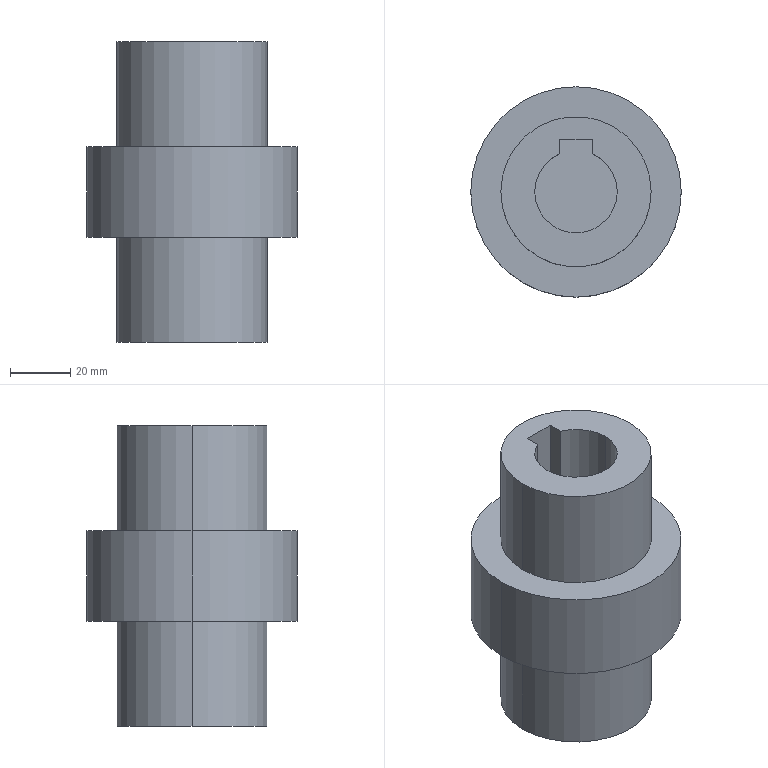Part | SolidWorks | features ICE 5, Extrusion 1 | 1 solid | 24 faces | box 70 x 70 x 100 mm | volume 224245 mm3 | plane 13 | cylinder 11 | commonest cylinder face diameters 50 x4 27.5 x3 25 x2 70 x2
STEP:
#1=CARTESIAN_POINT('',(-13.75,0.,25.));
#2=VERTEX_POINT('',#1);
#3=CARTESIAN_POINT('',(13.75,0.,25.));
#4=VERTEX_POINT('',#3);
#5=CARTESIAN_POINT('',(0.,0.,25.));
#6=DIRECTION('',(0.,0.,1.));
#7=DIRECTION('',(1.,0.,0.));
#8=AXIS2_PLACEMENT_3D('',#5,#6,#7);
#9=CIRCLE('',#8,13.75);
#10=EDGE_CURVE('',#2,#4,#9,.T.);
#11=ORIENTED_EDGE('',*,*,#10,.F.);
#12=CARTESIAN_POINT('',(-13.75,0.,50.));
#13=VERTEX_POINT('',#12);
#14=CARTESIAN_POINT('',(-13.75,0.,25.));
#15=DIRECTION('',(0.,0.,1.));
#16=VECTOR('',#15,1000.);
#17=LINE('',#14,#16);
#18=EDGE_CURVE('',#2,#13,#17,.T.);
#19=ORIENTED_EDGE('',*,*,#18,.T.);
#20=CARTESIAN_POINT('',(13.75,0.,50.));
#21=VERTEX_POINT('',#20);
#22=CARTESIAN_POINT('',(0.,0.,50.));
#23=DIRECTION('',(0.,0.,1.));
#24=DIRECTION('',(1.,0.,0.));
#25=AXIS2_PLACEMENT_3D('',#22,#23,#24);
#26=CIRCLE('',#25,13.75);
#27=EDGE_CURVE('',#13,#21,#26,.T.);
#28=ORIENTED_EDGE('',*,*,#27,.T.);
#29=CARTESIAN_POINT('',(13.75,0.,25.));
#30=DIRECTION('',(0.,0.,1.));
#31=VECTOR('',#30,1000.);
#32=LINE('',#29,#31);
#33=EDGE_CURVE('',#4,#21,#32,.T.);
#34=ORIENTED_EDGE('',*,*,#33,.F.);
#35=EDGE_LOOP('',(#11,#19,#28,#34));
#36=FACE_OUTER_BOUND('',#35,.T.);
#37=CARTESIAN_POINT('',(0.,0.,25.));
#38=DIRECTION('',(0.,0.,1.));
#39=DIRECTION('',(1.,0.,0.));
#40=AXIS2_PLACEMENT_3D('',#37,#38,#39);
#41=CYLINDRICAL_SURFACE('',#40,13.75);
#42=ADVANCED_FACE('',(#36),#41,.F.);
#43=CARTESIAN_POINT('',(5.385,12.652,25.));
#44=VERTEX_POINT('',#43);
#45=CARTESIAN_POINT('',(0.,0.,25.));
#46=DIRECTION('',(0.,0.,1.));
#47=DIRECTION('',(1.,0.,0.));
#48=AXIS2_PLACEMENT_3D('',#45,#46,#47);
#49=CIRCLE('',#48,13.75);
#50=EDGE_CURVE('',#4,#44,#49,.T.);
#51=ORIENTED_EDGE('',*,*,#50,.F.);
#52=ORIENTED_EDGE('',*,*,#33,.T.);
#53=CARTESIAN_POINT('',(5.385,12.652,50.));
#54=VERTEX_POINT('',#53);
#55=CARTESIAN_POINT('',(0.,0.,50.));
#56=DIRECTION('',(0.,0.,1.));
#57=DIRECTION('',(1.,0.,0.));
#58=AXIS2_PLACEMENT_3D('',#55,#56,#57);
#59=CIRCLE('',#58,13.75);
#60=EDGE_CURVE('',#21,#54,#59,.T.);
#61=ORIENTED_EDGE('',*,*,#60,.T.);
#62=CARTESIAN_POINT('',(5.385,12.652,25.));
#63=DIRECTION('',(0.,0.,1.));
#64=VECTOR('',#63,1000.);
#65=LINE('',#62,#64);
#66=EDGE_CURVE('',#44,#54,#65,.T.);
#67=ORIENTED_EDGE('',*,*,#66,.F.);
#68=EDGE_LOOP('',(#51,#52,#61,#67));
#69=FACE_OUTER_BOUND('',#68,.T.);
#70=CARTESIAN_POINT('',(0.,0.,25.));
#71=DIRECTION('',(0.,0.,1.));
#72=DIRECTION('',(1.,0.,0.));
#73=AXIS2_PLACEMENT_3D('',#70,#71,#72);
#74=CYLINDRICAL_SURFACE('',#73,13.75);
#75=ADVANCED_FACE('',(#69),#74,.F.);
#76=CARTESIAN_POINT('',(-25.,0.,-50.));
#77=VERTEX_POINT('',#76);
#78=CARTESIAN_POINT('',(25.,0.,-50.));
#79=VERTEX_POINT('',#78);
#80=CARTESIAN_POINT('',(0.,0.,-50.));
#81=DIRECTION('',(0.,0.,-1.));
#82=DIRECTION('',(-1.,0.,0.));
#83=AXIS2_PLACEMENT_3D('',#80,#81,#82);
#84=CIRCLE('',#83,25.);
#85=EDGE_CURVE('',#77,#79,#84,.T.);
#86=ORIENTED_EDGE('',*,*,#85,.F.);
#87=CARTESIAN_POINT('',(-25.,0.,-15.));
#88=VERTEX_POINT('',#87);
#89=CARTESIAN_POINT('',(-25.,0.,-50.));
#90=DIRECTION('',(0.,0.,1.));
#91=VECTOR('',#90,1000.);
#92=LINE('',#89,#91);
#93=EDGE_CURVE('',#77,#88,#92,.T.);
#94=ORIENTED_EDGE('',*,*,#93,.T.);
#95=CARTESIAN_POINT('',(25.,0.,-15.));
#96=VERTEX_POINT('',#95);
#97=CARTESIAN_POINT('',(0.,0.,-15.));
#98=DIRECTION('',(0.,0.,-1.));
#99=DIRECTION('',(-1.,0.,0.));
#100=AXIS2_PLACEMENT_3D('',#97,#98,#99);
#101=CIRCLE('',#100,25.);
#102=EDGE_CURVE('',#88,#96,#101,.T.);
#103=ORIENTED_EDGE('',*,*,#102,.T.);
#104=CARTESIAN_POINT('',(25.,0.,-50.));
#105=DIRECTION('',(0.,0.,1.));
#106=VECTOR('',#105,1000.);
#107=LINE('',#104,#106);
#108=EDGE_CURVE('',#79,#96,#107,.T.);
#109=ORIENTED_EDGE('',*,*,#108,.F.);
#110=EDGE_LOOP('',(#86,#94,#103,#109));
#111=FACE_OUTER_BOUND('',#110,.T.);
#112=CARTESIAN_POINT('',(0.,0.,-50.));
#113=DIRECTION('',(0.,0.,1.));
#114=DIRECTION('',(1.,0.,0.));
#115=AXIS2_PLACEMENT_3D('',#112,#113,#114);
#116=CYLINDRICAL_SURFACE('',#115,25.);
#117=ADVANCED_FACE('',(#111),#116,.T.);
#118=CARTESIAN_POINT('',(25.,0.,50.));
#119=VERTEX_POINT('',#118);
#120=CARTESIAN_POINT('',(-25.,0.,50.));
#121=VERTEX_POINT('',#120);
#122=CARTESIAN_POINT('',(0.,0.,50.));
#123=DIRECTION('',(0.,0.,1.));
#124=DIRECTION('',(1.,0.,0.));
#125=AXIS2_PLACEMENT_3D('',#122,#123,#124);
#126=CIRCLE('',#125,25.);
#127=EDGE_CURVE('',#119,#121,#126,.T.);
#128=ORIENTED_EDGE('',*,*,#127,.F.);
#129=CARTESIAN_POINT('',(25.,0.,15.));
#130=VERTEX_POINT('',#129);
#131=CARTESIAN_POINT('',(25.,0.,50.));
#132=DIRECTION('',(0.,0.,-1.));
#133=VECTOR('',#132,1000.);
#134=LINE('',#131,#133);
#135=EDGE_CURVE('',#119,#130,#134,.T.);
#136=ORIENTED_EDGE('',*,*,#135,.T.);
#137=CARTESIAN_POINT('',(-25.,0.,15.));
#138=VERTEX_POINT('',#137);
#139=CARTESIAN_POINT('',(0.,0.,15.));
#140=DIRECTION('',(0.,0.,1.));
#141=DIRECTION('',(1.,0.,0.));
#142=AXIS2_PLACEMENT_3D('',#139,#140,#141);
#143=CIRCLE('',#142,25.);
#144=EDGE_CURVE('',#130,#138,#143,.T.);
#145=ORIENTED_EDGE('',*,*,#144,.T.);
#146=CARTESIAN_POINT('',(-25.,0.,50.));
#147=DIRECTION('',(0.,0.,-1.));
#148=VECTOR('',#147,1000.);
#149=LINE('',#146,#148);
#150=EDGE_CURVE('',#121,#138,#149,.T.);
#151=ORIENTED_EDGE('',*,*,#150,.F.);
#152=EDGE_LOOP('',(#128,#136,#145,#151));
#153=FACE_OUTER_BOUND('',#152,.T.);
#154=CARTESIAN_POINT('',(0.,0.,50.));
#155=DIRECTION('',(0.,0.,-1.));
#156=DIRECTION('',(-1.,0.,0.));
#157=AXIS2_PLACEMENT_3D('',#154,#155,#156);
#158=CYLINDRICAL_SURFACE('',#157,25.);
#159=ADVANCED_FACE('',(#153),#158,.T.);
#160=CARTESIAN_POINT('',(35.,0.,15.));
#161=VERTEX_POINT('',#160);
#162=CARTESIAN_POINT('',(-35.,0.,15.));
#163=VERTEX_POINT('',#162);
#164=CARTESIAN_POINT('',(0.,0.,15.));
#165=DIRECTION('',(0.,0.,1.));
#166=DIRECTION('',(1.,0.,0.));
#167=AXIS2_PLACEMENT_3D('',#164,#165,#166);
#168=CIRCLE('',#167,35.);
#169=EDGE_CURVE('',#161,#163,#168,.T.);
#170=ORIENTED_EDGE('',*,*,#169,.F.);
#171=CARTESIAN_POINT('',(35.,0.,-15.));
#172=VERTEX_POINT('',#171);
#173=CARTESIAN_POINT('',(35.,0.,15.));
#174=DIRECTION('',(0.,0.,-1.));
#175=VECTOR('',#174,1000.);
#176=LINE('',#173,#175);
#177=EDGE_CURVE('',#161,#172,#176,.T.);
#178=ORIENTED_EDGE('',*,*,#177,.T.);
#179=CARTESIAN_POINT('',(-35.,0.,-15.));
#180=VERTEX_POINT('',#179);
#181=CARTESIAN_POINT('',(0.,0.,-15.));
#182=DIRECTION('',(0.,0.,1.));
#183=DIRECTION('',(1.,0.,0.));
#184=AXIS2_PLACEMENT_3D('',#181,#182,#183);
#185=CIRCLE('',#184,35.);
#186=EDGE_CURVE('',#172,#180,#185,.T.);
#187=ORIENTED_EDGE('',*,*,#186,.T.);
#188=CARTESIAN_POINT('',(-35.,0.,15.));
#189=DIRECTION('',(0.,0.,-1.));
#190=VECTOR('',#189,1000.);
#191=LINE('',#188,#190);
#192=EDGE_CURVE('',#163,#180,#191,.T.);
#193=ORIENTED_EDGE('',*,*,#192,.F.);
#194=EDGE_LOOP('',(#170,#178,#187,#193));
#195=FACE_OUTER_BOUND('',#194,.T.);
#196=CARTESIAN_POINT('',(0.,0.,15.));
#197=DIRECTION('',(0.,0.,-1.));
#198=DIRECTION('',(-1.,0.,0.));
#199=AXIS2_PLACEMENT_3D('',#196,#197,#198);
#200=CYLINDRICAL_SURFACE('',#199,35.);
#201=ADVANCED_FACE('',(#195),#200,.T.);
#202=CARTESIAN_POINT('',(12.5,0.,-25.));
#203=VERTEX_POINT('',#202);
#204=CARTESIAN_POINT('',(-12.5,0.,-25.));
#205=VERTEX_POINT('',#204);
#206=CARTESIAN_POINT('',(0.,0.,-25.));
#207=DIRECTION('',(0.,0.,-1.));
#208=DIRECTION('',(-1.,0.,0.));
#209=AXIS2_PLACEMENT_3D('',#206,#207,#208);
#210=CIRCLE('',#209,12.5);
#211=EDGE_CURVE('',#203,#205,#210,.T.);
#212=ORIENTED_EDGE('',*,*,#211,.F.);
#213=CARTESIAN_POINT('',(12.5,0.,-50.));
#214=VERTEX_POINT('',#213);
#215=CARTESIAN_POINT('',(12.5,0.,-25.));
#216=DIRECTION('',(0.,0.,-1.));
#217=VECTOR('',#216,1000.);
#218=LINE('',#215,#217);
#219=EDGE_CURVE('',#203,#214,#218,.T.);
#220=ORIENTED_EDGE('',*,*,#219,.T.);
#221=CARTESIAN_POINT('',(-12.5,0.,-50.));
#222=VERTEX_POINT('',#221);
#223=CARTESIAN_POINT('',(0.,0.,-50.));
#224=DIRECTION('',(0.,0.,-1.));
#225=DIRECTION('',(-1.,0.,0.));
#226=AXIS2_PLACEMENT_3D('',#223,#224,#225);
#227=CIRCLE('',#226,12.5);
#228=EDGE_CURVE('',#214,#222,#227,.T.);
#229=ORIENTED_EDGE('',*,*,#228,.T.);
#230=CARTESIAN_POINT('',(-12.5,0.,-25.));
#231=DIRECTION('',(0.,0.,-1.));
#232=VECTOR('',#231,1000.);
#233=LINE('',#230,#232);
#234=EDGE_CURVE('',#205,#222,#233,.T.);
#235=ORIENTED_EDGE('',*,*,#234,.F.);
#236=EDGE_LOOP('',(#212,#220,#229,#235));
#237=FACE_OUTER_BOUND('',#236,.T.);
#238=CARTESIAN_POINT('',(0.,0.,-25.));
#239=DIRECTION('',(0.,0.,-1.));
#240=DIRECTION('',(-1.,0.,0.));
#241=AXIS2_PLACEMENT_3D('',#238,#239,#240);
#242=CYLINDRICAL_SURFACE('',#241,12.5);
#243=ADVANCED_FACE('',(#237),#242,.F.);
#244=CARTESIAN_POINT('',(0.,0.,-50.));
#245=DIRECTION('',(0.,0.,-1.));
#246=DIRECTION('',(-1.,0.,0.));
#247=AXIS2_PLACEMENT_3D('',#244,#245,#246);
#248=CIRCLE('',#247,25.);
#249=EDGE_CURVE('',#79,#77,#248,.T.);
#250=ORIENTED_EDGE('',*,*,#249,.T.);
#251=ORIENTED_EDGE('',*,*,#85,.T.);
#252=EDGE_LOOP('',(#250,#251));
#253=FACE_OUTER_BOUND('',#252,.T.);
#254=CARTESIAN_POINT('',(5.,15.,-50.));
#255=VERTEX_POINT('',#254);
#256=CARTESIAN_POINT('',(-5.,15.,-50.));
#257=VERTEX_POINT('',#256);
#258=CARTESIAN_POINT('',(0.,15.,-50.));
#259=DIRECTION('',(-1.,0.,0.));
#260=VECTOR('',#259,1000.);
#261=LINE('',#258,#260);
#262=EDGE_CURVE('',#255,#257,#261,.T.);
#263=ORIENTED_EDGE('',*,*,#262,.T.);
#264=CARTESIAN_POINT('',(-5.,11.456,-50.));
#265=VERTEX_POINT('',#264);
#266=CARTESIAN_POINT('',(-5.,0.,-50.));
#267=DIRECTION('',(0.,-1.,0.));
#268=VECTOR('',#267,1000.);
#269=LINE('',#266,#268);
#270=EDGE_CURVE('',#257,#265,#269,.T.);
#271=ORIENTED_EDGE('',*,*,#270,.T.);
#272=CARTESIAN_POINT('',(0.,0.,-50.));
#273=DIRECTION('',(0.,0.,-1.));
#274=DIRECTION('',(-1.,0.,0.));
#275=AXIS2_PLACEMENT_3D('',#272,#273,#274);
#276=CIRCLE('',#275,12.5);
#277=EDGE_CURVE('',#222,#265,#276,.T.);
#278=ORIENTED_EDGE('',*,*,#277,.F.);
#279=ORIENTED_EDGE('',*,*,#228,.F.);
#280=CARTESIAN_POINT('',(5.,11.456,-50.));
#281=VERTEX_POINT('',#280);
#282=CARTESIAN_POINT('',(0.,0.,-50.));
#283=DIRECTION('',(0.,0.,-1.));
#284=DIRECTION('',(-1.,0.,0.));
#285=AXIS2_PLACEMENT_3D('',#282,#283,#284);
#286=CIRCLE('',#285,12.5);
#287=EDGE_CURVE('',#281,#214,#286,.T.);
#288=ORIENTED_EDGE('',*,*,#287,.F.);
#289=CARTESIAN_POINT('',(5.,0.,-50.));
#290=DIRECTION('',(0.,-1.,0.));
#291=VECTOR('',#290,1000.);
#292=LINE('',#289,#291);
#293=EDGE_CURVE('',#255,#281,#292,.T.);
#294=ORIENTED_EDGE('',*,*,#293,.F.);
#295=EDGE_LOOP('',(#263,#271,#278,#279,#288,#294));
#296=FACE_BOUND('',#295,.T.);
#297=CARTESIAN_POINT('',(0.,0.,-50.));
#298=DIRECTION('',(0.,0.,-1.));
#299=DIRECTION('',(-1.,0.,0.));
#300=AXIS2_PLACEMENT_3D('',#297,#298,#299);
#301=PLANE('',#300);
#302=ADVANCED_FACE('',(#253,#296),#301,.T.);
#303=ORIENTED_EDGE('',*,*,#219,.F.);
#304=CARTESIAN_POINT('',(0.,0.,-25.));
#305=DIRECTION('',(0.,0.,-1.));
#306=DIRECTION('',(-1.,0.,0.));
#307=AXIS2_PLACEMENT_3D('',#304,#305,#306);
#308=CIRCLE('',#307,12.5);
#309=EDGE_CURVE('',#205,#203,#308,.T.);
#310=ORIENTED_EDGE('',*,*,#309,.F.);
#311=ORIENTED_EDGE('',*,*,#234,.T.);
#312=ORIENTED_EDGE('',*,*,#277,.T.);
#313=CARTESIAN_POINT('',(-5.,11.456,-35.));
#314=VERTEX_POINT('',#313);
#315=CARTESIAN_POINT('',(-5.,11.456,-35.));
#316=DIRECTION('',(0.,0.,-1.));
#317=VECTOR('',#316,1000.);
#318=LINE('',#315,#317);
#319=EDGE_CURVE('',#314,#265,#318,.T.);
#320=ORIENTED_EDGE('',*,*,#319,.F.);
#321=CARTESIAN_POINT('',(5.,11.456,-35.));
#322=VERTEX_POINT('',#321);
#323=CARTESIAN_POINT('',(0.,0.,-35.));
#324=DIRECTION('',(0.,0.,-1.));
#325=DIRECTION('',(-1.,0.,0.));
#326=AXIS2_PLACEMENT_3D('',#323,#324,#325);
#327=CIRCLE('',#326,12.5);
#328=EDGE_CURVE('',#314,#322,#327,.T.);
#329=ORIENTED_EDGE('',*,*,#328,.T.);
#330=CARTESIAN_POINT('',(5.,11.456,-35.));
#331=DIRECTION('',(0.,0.,-1.));
#332=VECTOR('',#331,1000.);
#333=LINE('',#330,#332);
#334=EDGE_CURVE('',#322,#281,#333,.T.);
#335=ORIENTED_EDGE('',*,*,#334,.T.);
#336=ORIENTED_EDGE('',*,*,#287,.T.);
#337=EDGE_LOOP('',(#303,#310,#311,#312,#320,#329,#335,#336));
#338=FACE_OUTER_BOUND('',#337,.T.);
#339=CARTESIAN_POINT('',(0.,0.,-25.));
#340=DIRECTION('',(0.,0.,-1.));
#341=DIRECTION('',(-1.,0.,0.));
#342=AXIS2_PLACEMENT_3D('',#339,#340,#341);
#343=CYLINDRICAL_SURFACE('',#342,12.5);
#344=ADVANCED_FACE('',(#338),#343,.F.);
#345=ORIENTED_EDGE('',*,*,#177,.F.);
#346=CARTESIAN_POINT('',(0.,0.,15.));
#347=DIRECTION('',(0.,0.,1.));
#348=DIRECTION('',(1.,0.,0.));
#349=AXIS2_PLACEMENT_3D('',#346,#347,#348);
#350=CIRCLE('',#349,35.);
#351=EDGE_CURVE('',#163,#161,#350,.T.);
#352=ORIENTED_EDGE('',*,*,#351,.F.);
#353=ORIENTED_EDGE('',*,*,#192,.T.);
#354=CARTESIAN_POINT('',(0.,0.,-15.));
#355=DIRECTION('',(0.,0.,1.));
#356=DIRECTION('',(1.,0.,0.));
#357=AXIS2_PLACEMENT_3D('',#354,#355,#356);
#358=CIRCLE('',#357,35.);
#359=EDGE_CURVE('',#180,#172,#358,.T.);
#360=ORIENTED_EDGE('',*,*,#359,.T.);
#361=EDGE_LOOP('',(#345,#352,#353,#360));
#362=FACE_OUTER_BOUND('',#361,.T.);
#363=CARTESIAN_POINT('',(0.,0.,15.));
#364=DIRECTION('',(0.,0.,-1.));
#365=DIRECTION('',(-1.,0.,0.));
#366=AXIS2_PLACEMENT_3D('',#363,#364,#365);
#367=CYLINDRICAL_SURFACE('',#366,35.);
#368=ADVANCED_FACE('',(#362),#367,.T.);
#369=CARTESIAN_POINT('',(0.,0.,15.));
#370=DIRECTION('',(0.,0.,1.));
#371=DIRECTION('',(1.,0.,0.));
#372=AXIS2_PLACEMENT_3D('',#369,#370,#371);
#373=CIRCLE('',#372,25.);
#374=EDGE_CURVE('',#138,#130,#373,.T.);
#375=ORIENTED_EDGE('',*,*,#374,.F.);
#376=ORIENTED_EDGE('',*,*,#144,.F.);
#377=EDGE_LOOP('',(#375,#376));
#378=FACE_BOUND('',#377,.T.);
#379=ORIENTED_EDGE('',*,*,#351,.T.);
#380=ORIENTED_EDGE('',*,*,#169,.T.);
#381=EDGE_LOOP('',(#379,#380));
#382=FACE_OUTER_BOUND('',#381,.T.);
#383=CARTESIAN_POINT('',(0.,0.,15.));
#384=DIRECTION('',(0.,0.,1.));
#385=DIRECTION('',(1.,0.,0.));
#386=AXIS2_PLACEMENT_3D('',#383,#384,#385);
#387=PLANE('',#386);
#388=ADVANCED_FACE('',(#378,#382),#387,.T.);
#389=CARTESIAN_POINT('',(0.,0.,-15.));
#390=DIRECTION('',(0.,0.,-1.));
#391=DIRECTION('',(-1.,0.,0.));
#392=AXIS2_PLACEMENT_3D('',#389,#390,#391);
#393=CIRCLE('',#392,25.);
#394=EDGE_CURVE('',#96,#88,#393,.T.);
#395=ORIENTED_EDGE('',*,*,#394,.F.);
#396=ORIENTED_EDGE('',*,*,#102,.F.);
#397=EDGE_LOOP('',(#395,#396));
#398=FACE_BOUND('',#397,.T.);
#399=ORIENTED_EDGE('',*,*,#359,.F.);
#400=ORIENTED_EDGE('',*,*,#186,.F.);
#401=EDGE_LOOP('',(#399,#400));
#402=FACE_OUTER_BOUND('',#401,.T.);
#403=CARTESIAN_POINT('',(0.,0.,-15.));
#404=DIRECTION('',(0.,0.,1.));
#405=DIRECTION('',(1.,0.,0.));
#406=AXIS2_PLACEMENT_3D('',#403,#404,#405);
#407=PLANE('',#406);
#408=ADVANCED_FACE('',(#398,#402),#407,.F.);
#409=ORIENTED_EDGE('',*,*,#135,.F.);
#410=CARTESIAN_POINT('',(0.,0.,50.));
#411=DIRECTION('',(0.,0.,1.));
#412=DIRECTION('',(1.,0.,0.));
#413=AXIS2_PLACEMENT_3D('',#410,#411,#412);
#414=CIRCLE('',#413,25.);
#415=EDGE_CURVE('',#121,#119,#414,.T.);
#416=ORIENTED_EDGE('',*,*,#415,.F.);
#417=ORIENTED_EDGE('',*,*,#150,.T.);
#418=ORIENTED_EDGE('',*,*,#374,.T.);
#419=EDGE_LOOP('',(#409,#416,#417,#418));
#420=FACE_OUTER_BOUND('',#419,.T.);
#421=CARTESIAN_POINT('',(0.,0.,50.));
#422=DIRECTION('',(0.,0.,-1.));
#423=DIRECTION('',(-1.,0.,0.));
#424=AXIS2_PLACEMENT_3D('',#421,#422,#423);
#425=CYLINDRICAL_SURFACE('',#424,25.);
#426=ADVANCED_FACE('',(#420),#425,.T.);
#427=CARTESIAN_POINT('',(-5.385,17.5,50.));
#428=VERTEX_POINT('',#427);
#429=CARTESIAN_POINT('',(-5.385,12.652,50.));
#430=VERTEX_POINT('',#429);
#431=CARTESIAN_POINT('',(-5.385,0.,50.));
#432=DIRECTION('',(0.,-1.,0.));
#433=VECTOR('',#432,1000.);
#434=LINE('',#431,#433);
#435=EDGE_CURVE('',#428,#430,#434,.T.);
#436=ORIENTED_EDGE('',*,*,#435,.F.);
#437=CARTESIAN_POINT('',(5.385,17.5,50.));
#438=VERTEX_POINT('',#437);
#439=CARTESIAN_POINT('',(0.,17.5,50.));
#440=DIRECTION('',(1.,0.,0.));
#441=VECTOR('',#440,1000.);
#442=LINE('',#439,#441);
#443=EDGE_CURVE('',#428,#438,#442,.T.);
#444=ORIENTED_EDGE('',*,*,#443,.T.);
#445=CARTESIAN_POINT('',(5.385,0.,50.));
#446=DIRECTION('',(0.,-1.,0.));
#447=VECTOR('',#446,1000.);
#448=LINE('',#445,#447);
#449=EDGE_CURVE('',#438,#54,#448,.T.);
#450=ORIENTED_EDGE('',*,*,#449,.T.);
#451=ORIENTED_EDGE('',*,*,#60,.F.);
#452=ORIENTED_EDGE('',*,*,#27,.F.);
#453=CARTESIAN_POINT('',(0.,0.,50.));
#454=DIRECTION('',(0.,0.,1.));
#455=DIRECTION('',(1.,0.,0.));
#456=AXIS2_PLACEMENT_3D('',#453,#454,#455);
#457=CIRCLE('',#456,13.75);
#458=EDGE_CURVE('',#430,#13,#457,.T.);
#459=ORIENTED_EDGE('',*,*,#458,.F.);
#460=EDGE_LOOP('',(#436,#444,#450,#451,#452,#459));
#461=FACE_BOUND('',#460,.T.);
#462=ORIENTED_EDGE('',*,*,#415,.T.);
#463=ORIENTED_EDGE('',*,*,#127,.T.);
#464=EDGE_LOOP('',(#462,#463));
#465=FACE_OUTER_BOUND('',#464,.T.);
#466=CARTESIAN_POINT('',(0.,0.,50.));
#467=DIRECTION('',(0.,0.,1.));
#468=DIRECTION('',(1.,0.,0.));
#469=AXIS2_PLACEMENT_3D('',#466,#467,#468);
#470=PLANE('',#469);
#471=ADVANCED_FACE('',(#461,#465),#470,.T.);
#472=ORIENTED_EDGE('',*,*,#93,.F.);
#473=ORIENTED_EDGE('',*,*,#249,.F.);
#474=ORIENTED_EDGE('',*,*,#108,.T.);
#475=ORIENTED_EDGE('',*,*,#394,.T.);
#476=EDGE_LOOP('',(#472,#473,#474,#475));
#477=FACE_OUTER_BOUND('',#476,.T.);
#478=CARTESIAN_POINT('',(0.,0.,-50.));
#479=DIRECTION('',(0.,0.,1.));
#480=DIRECTION('',(1.,0.,0.));
#481=AXIS2_PLACEMENT_3D('',#478,#479,#480);
#482=CYLINDRICAL_SURFACE('',#481,25.);
#483=ADVANCED_FACE('',(#477),#482,.T.);
#484=ORIENTED_EDGE('',*,*,#435,.T.);
#485=CARTESIAN_POINT('',(-5.385,12.652,25.));
#486=VERTEX_POINT('',#485);
#487=CARTESIAN_POINT('',(-5.385,12.652,25.));
#488=DIRECTION('',(0.,0.,1.));
#489=VECTOR('',#488,1000.);
#490=LINE('',#487,#489);
#491=EDGE_CURVE('',#486,#430,#490,.T.);
#492=ORIENTED_EDGE('',*,*,#491,.F.);
#493=CARTESIAN_POINT('',(-5.385,17.5,25.));
#494=VERTEX_POINT('',#493);
#495=CARTESIAN_POINT('',(-5.385,17.5,25.));
#496=DIRECTION('',(0.,-1.,0.));
#497=VECTOR('',#496,1000.);
#498=LINE('',#495,#497);
#499=EDGE_CURVE('',#494,#486,#498,.T.);
#500=ORIENTED_EDGE('',*,*,#499,.F.);
#501=CARTESIAN_POINT('',(-5.385,17.5,25.));
#502=DIRECTION('',(0.,0.,1.));
#503=VECTOR('',#502,1000.);
#504=LINE('',#501,#503);
#505=EDGE_CURVE('',#494,#428,#504,.T.);
#506=ORIENTED_EDGE('',*,*,#505,.T.);
#507=EDGE_LOOP('',(#484,#492,#500,#506));
#508=FACE_OUTER_BOUND('',#507,.T.);
#509=CARTESIAN_POINT('',(-5.385,17.5,25.));
#510=DIRECTION('',(-1.,0.,0.));
#511=DIRECTION('',(0.,0.,1.));
#512=AXIS2_PLACEMENT_3D('',#509,#510,#511);
#513=PLANE('',#512);
#514=ADVANCED_FACE('',(#508),#513,.F.);
#515=ORIENTED_EDGE('',*,*,#505,.F.);
#516=CARTESIAN_POINT('',(5.385,17.5,25.));
#517=VERTEX_POINT('',#516);
#518=CARTESIAN_POINT('',(-5.385,17.5,25.));
#519=DIRECTION('',(1.,0.,0.));
#520=VECTOR('',#519,1000.);
#521=LINE('',#518,#520);
#522=EDGE_CURVE('',#494,#517,#521,.T.);
#523=ORIENTED_EDGE('',*,*,#522,.T.);
#524=CARTESIAN_POINT('',(5.385,17.5,25.));
#525=DIRECTION('',(0.,0.,1.));
#526=VECTOR('',#525,1000.);
#527=LINE('',#524,#526);
#528=EDGE_CURVE('',#517,#438,#527,.T.);
#529=ORIENTED_EDGE('',*,*,#528,.T.);
#530=ORIENTED_EDGE('',*,*,#443,.F.);
#531=EDGE_LOOP('',(#515,#523,#529,#530));
#532=FACE_OUTER_BOUND('',#531,.T.);
#533=CARTESIAN_POINT('',(-5.385,17.5,25.));
#534=DIRECTION('',(0.,-1.,0.));
#535=DIRECTION('',(0.,0.,-1.));
#536=AXIS2_PLACEMENT_3D('',#533,#534,#535);
#537=PLANE('',#536);
#538=ADVANCED_FACE('',(#532),#537,.T.);
#539=ORIENTED_EDGE('',*,*,#528,.F.);
#540=CARTESIAN_POINT('',(5.385,17.5,25.));
#541=DIRECTION('',(0.,-1.,0.));
#542=VECTOR('',#541,1000.);
#543=LINE('',#540,#542);
#544=EDGE_CURVE('',#517,#44,#543,.T.);
#545=ORIENTED_EDGE('',*,*,#544,.T.);
#546=ORIENTED_EDGE('',*,*,#66,.T.);
#547=ORIENTED_EDGE('',*,*,#449,.F.);
#548=EDGE_LOOP('',(#539,#545,#546,#547));
#549=FACE_OUTER_BOUND('',#548,.T.);
#550=CARTESIAN_POINT('',(5.385,17.5,25.));
#551=DIRECTION('',(-1.,0.,0.));
#552=DIRECTION('',(0.,0.,1.));
#553=AXIS2_PLACEMENT_3D('',#550,#551,#552);
#554=PLANE('',#553);
#555=ADVANCED_FACE('',(#549),#554,.T.);
#556=ORIENTED_EDGE('',*,*,#18,.F.);
#557=CARTESIAN_POINT('',(0.,0.,25.));
#558=DIRECTION('',(0.,0.,1.));
#559=DIRECTION('',(1.,0.,0.));
#560=AXIS2_PLACEMENT_3D('',#557,#558,#559);
#561=CIRCLE('',#560,13.75);
#562=EDGE_CURVE('',#486,#2,#561,.T.);
#563=ORIENTED_EDGE('',*,*,#562,.F.);
#564=ORIENTED_EDGE('',*,*,#491,.T.);
#565=ORIENTED_EDGE('',*,*,#458,.T.);
#566=EDGE_LOOP('',(#556,#563,#564,#565));
#567=FACE_OUTER_BOUND('',#566,.T.);
#568=CARTESIAN_POINT('',(0.,0.,25.));
#569=DIRECTION('',(0.,0.,1.));
#570=DIRECTION('',(1.,0.,0.));
#571=AXIS2_PLACEMENT_3D('',#568,#569,#570);
#572=CYLINDRICAL_SURFACE('',#571,13.75);
#573=ADVANCED_FACE('',(#567),#572,.F.);
#574=ORIENTED_EDGE('',*,*,#499,.T.);
#575=ORIENTED_EDGE('',*,*,#562,.T.);
#576=ORIENTED_EDGE('',*,*,#10,.T.);
#577=ORIENTED_EDGE('',*,*,#50,.T.);
#578=ORIENTED_EDGE('',*,*,#544,.F.);
#579=ORIENTED_EDGE('',*,*,#522,.F.);
#580=EDGE_LOOP('',(#574,#575,#576,#577,#578,#579));
#581=FACE_OUTER_BOUND('',#580,.T.);
#582=CARTESIAN_POINT('',(0.,0.,25.));
#583=DIRECTION('',(0.,0.,1.));
#584=DIRECTION('',(1.,0.,0.));
#585=AXIS2_PLACEMENT_3D('',#582,#583,#584);
#586=PLANE('',#585);
#587=ADVANCED_FACE('',(#581),#586,.T.);
#588=ORIENTED_EDGE('',*,*,#309,.T.);
#589=ORIENTED_EDGE('',*,*,#211,.T.);
#590=EDGE_LOOP('',(#588,#589));
#591=FACE_OUTER_BOUND('',#590,.T.);
#592=CARTESIAN_POINT('',(0.,0.,-25.));
#593=DIRECTION('',(0.,0.,-1.));
#594=DIRECTION('',(-1.,0.,0.));
#595=AXIS2_PLACEMENT_3D('',#592,#593,#594);
#596=PLANE('',#595);
#597=ADVANCED_FACE('',(#591),#596,.T.);
#598=CARTESIAN_POINT('',(5.,15.,-35.));
#599=VERTEX_POINT('',#598);
#600=CARTESIAN_POINT('',(5.,15.,-35.));
#601=DIRECTION('',(0.,0.,-1.));
#602=VECTOR('',#601,1000.);
#603=LINE('',#600,#602);
#604=EDGE_CURVE('',#599,#255,#603,.T.);
#605=ORIENTED_EDGE('',*,*,#604,.F.);
#606=CARTESIAN_POINT('',(-5.,15.,-35.));
#607=VERTEX_POINT('',#606);
#608=CARTESIAN_POINT('',(5.,15.,-35.));
#609=DIRECTION('',(-1.,0.,0.));
#610=VECTOR('',#609,1000.);
#611=LINE('',#608,#610);
#612=EDGE_CURVE('',#599,#607,#611,.T.);
#613=ORIENTED_EDGE('',*,*,#612,.T.);
#614=CARTESIAN_POINT('',(-5.,15.,-35.));
#615=DIRECTION('',(0.,0.,-1.));
#616=VECTOR('',#615,1000.);
#617=LINE('',#614,#616);
#618=EDGE_CURVE('',#607,#257,#617,.T.);
#619=ORIENTED_EDGE('',*,*,#618,.T.);
#620=ORIENTED_EDGE('',*,*,#262,.F.);
#621=EDGE_LOOP('',(#605,#613,#619,#620));
#622=FACE_OUTER_BOUND('',#621,.T.);
#623=CARTESIAN_POINT('',(5.,15.,-35.));
#624=DIRECTION('',(0.,-1.,0.));
#625=DIRECTION('',(0.,0.,-1.));
#626=AXIS2_PLACEMENT_3D('',#623,#624,#625);
#627=PLANE('',#626);
#628=ADVANCED_FACE('',(#622),#627,.T.);
#629=ORIENTED_EDGE('',*,*,#618,.F.);
#630=CARTESIAN_POINT('',(-5.,15.,-35.));
#631=DIRECTION('',(0.,-1.,0.));
#632=VECTOR('',#631,1000.);
#633=LINE('',#630,#632);
#634=EDGE_CURVE('',#607,#314,#633,.T.);
#635=ORIENTED_EDGE('',*,*,#634,.T.);
#636=ORIENTED_EDGE('',*,*,#319,.T.);
#637=ORIENTED_EDGE('',*,*,#270,.F.);
#638=EDGE_LOOP('',(#629,#635,#636,#637));
#639=FACE_OUTER_BOUND('',#638,.T.);
#640=CARTESIAN_POINT('',(-5.,15.,-35.));
#641=DIRECTION('',(1.,0.,0.));
#642=DIRECTION('',(0.,0.,-1.));
#643=AXIS2_PLACEMENT_3D('',#640,#641,#642);
#644=PLANE('',#643);
#645=ADVANCED_FACE('',(#639),#644,.T.);
#646=ORIENTED_EDGE('',*,*,#293,.T.);
#647=ORIENTED_EDGE('',*,*,#334,.F.);
#648=CARTESIAN_POINT('',(5.,15.,-35.));
#649=DIRECTION('',(0.,-1.,0.));
#650=VECTOR('',#649,1000.);
#651=LINE('',#648,#650);
#652=EDGE_CURVE('',#599,#322,#651,.T.);
#653=ORIENTED_EDGE('',*,*,#652,.F.);
#654=ORIENTED_EDGE('',*,*,#604,.T.);
#655=EDGE_LOOP('',(#646,#647,#653,#654));
#656=FACE_OUTER_BOUND('',#655,.T.);
#657=CARTESIAN_POINT('',(5.,15.,-35.));
#658=DIRECTION('',(1.,0.,0.));
#659=DIRECTION('',(0.,0.,-1.));
#660=AXIS2_PLACEMENT_3D('',#657,#658,#659);
#661=PLANE('',#660);
#662=ADVANCED_FACE('',(#656),#661,.F.);
#663=ORIENTED_EDGE('',*,*,#612,.F.);
#664=ORIENTED_EDGE('',*,*,#652,.T.);
#665=ORIENTED_EDGE('',*,*,#328,.F.);
#666=ORIENTED_EDGE('',*,*,#634,.F.);
#667=EDGE_LOOP('',(#663,#664,#665,#666));
#668=FACE_OUTER_BOUND('',#667,.T.);
#669=CARTESIAN_POINT('',(0.,0.,-35.));
#670=DIRECTION('',(0.,0.,-1.));
#671=DIRECTION('',(-1.,0.,0.));
#672=AXIS2_PLACEMENT_3D('',#669,#670,#671);
#673=PLANE('',#672);
#674=ADVANCED_FACE('',(#668),#673,.T.);
#675=CLOSED_SHELL('',(#42,#75,#117,#159,#201,#243,#302,#344,#368,#388,#408,#426,#471,#483,#514,#538,#555,#573,#587,#597,#628,#645,#662,#674));
#676=MANIFOLD_SOLID_BREP('',#675);
#677=CARTESIAN_POINT('',(0.,0.,0.));
#678=DIRECTION('',(0.,0.,1.));
#679=DIRECTION('',(1.,0.,0.));
#680=AXIS2_PLACEMENT_3D('',#677,#678,#679);
#681=(LENGTH_UNIT()NAMED_UNIT(*)SI_UNIT(.MILLI.,.METRE.));
#682=UNCERTAINTY_MEASURE_WITH_UNIT(LENGTH_MEASURE(0.00001),#681,'','');
#683=(NAMED_UNIT(*)PLANE_ANGLE_UNIT()SI_UNIT($,.RADIAN.));
#684=(NAMED_UNIT(*)SI_UNIT($,.STERADIAN.)SOLID_ANGLE_UNIT());
#685=(GEOMETRIC_REPRESENTATION_CONTEXT(3)GLOBAL_UNCERTAINTY_ASSIGNED_CONTEXT((#682))GLOBAL_UNIT_ASSIGNED_CONTEXT((#681,#683,#684))REPRESENTATION_CONTEXT('',''));
#686=ADVANCED_BREP_SHAPE_REPRESENTATION('',(#676,#680),#685);